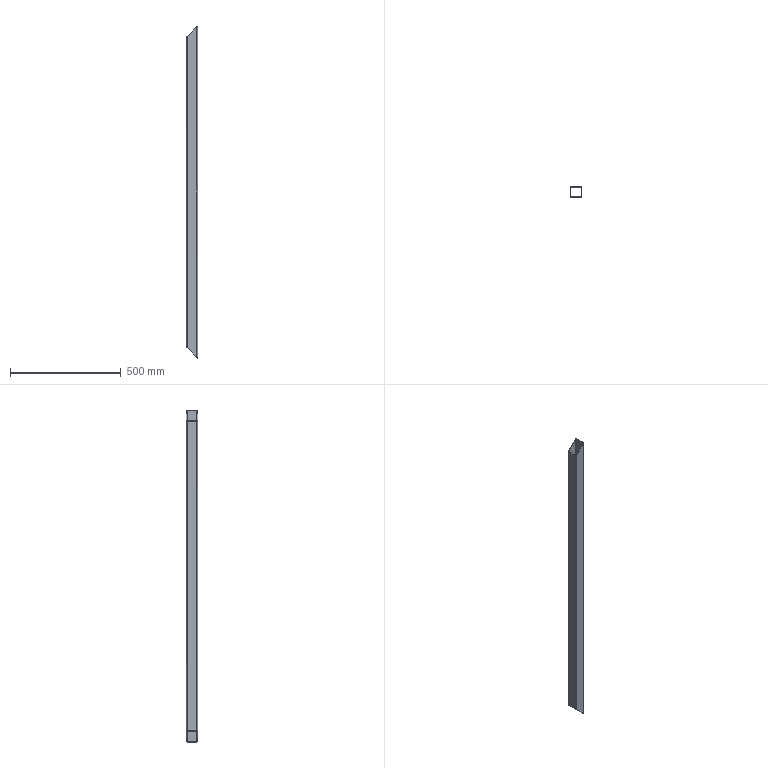Part | SolidWorks | features BaseBody 1 | 1 solid | 18 faces | box 50 x 50 x 1498 mm | volume 541116 mm3 | plane 10 | cylinder 8 | commonest cylinder face diameters 4 x4 8 x4
STEP:
#1=CARTESIAN_POINT('',(-25.,21.,699.));
#2=VERTEX_POINT('',#1);
#3=CARTESIAN_POINT('',(-25.,21.,-699.));
#4=VERTEX_POINT('',#3);
#5=CARTESIAN_POINT('',(-25.,21.,749.));
#6=DIRECTION('',(0.,0.,-1.));
#7=VECTOR('',#6,1000.);
#8=LINE('',#5,#7);
#9=EDGE_CURVE('',#2,#4,#8,.T.);
#10=ORIENTED_EDGE('',*,*,#9,.T.);
#11=CARTESIAN_POINT('',(-25.,-21.,-699.));
#12=VERTEX_POINT('',#11);
#13=CARTESIAN_POINT('',(-25.,-25.,-699.));
#14=DIRECTION('',(0.,1.,0.));
#15=VECTOR('',#14,1000.);
#16=LINE('',#13,#15);
#17=EDGE_CURVE('',#12,#4,#16,.T.);
#18=ORIENTED_EDGE('',*,*,#17,.F.);
#19=CARTESIAN_POINT('',(-25.,-21.,699.));
#20=VERTEX_POINT('',#19);
#21=CARTESIAN_POINT('',(-25.,-21.,749.));
#22=DIRECTION('',(0.,0.,-1.));
#23=VECTOR('',#22,1000.);
#24=LINE('',#21,#23);
#25=EDGE_CURVE('',#20,#12,#24,.T.);
#26=ORIENTED_EDGE('',*,*,#25,.F.);
#27=CARTESIAN_POINT('',(-25.,-25.,699.));
#28=DIRECTION('',(0.,1.,0.));
#29=VECTOR('',#28,1000.);
#30=LINE('',#27,#29);
#31=EDGE_CURVE('',#20,#2,#30,.T.);
#32=ORIENTED_EDGE('',*,*,#31,.T.);
#33=EDGE_LOOP('',(#10,#18,#26,#32));
#34=FACE_OUTER_BOUND('',#33,.T.);
#35=CARTESIAN_POINT('',(-25.,21.,749.));
#36=DIRECTION('',(1.,0.,0.));
#37=DIRECTION('',(0.,1.,0.));
#38=AXIS2_PLACEMENT_3D('',#35,#36,#37);
#39=PLANE('',#38);
#40=ADVANCED_FACE('',(#34),#39,.F.);
#41=CARTESIAN_POINT('',(-21.,25.,703.));
#42=VERTEX_POINT('',#41);
#43=CARTESIAN_POINT('',(-21.,25.,-703.));
#44=VERTEX_POINT('',#43);
#45=CARTESIAN_POINT('',(-21.,25.,749.));
#46=DIRECTION('',(0.,0.,-1.));
#47=VECTOR('',#46,1000.);
#48=LINE('',#45,#47);
#49=EDGE_CURVE('',#42,#44,#48,.T.);
#50=ORIENTED_EDGE('',*,*,#49,.T.);
#51=CARTESIAN_POINT('',(-21.,25.,-703.));
#52=CARTESIAN_POINT('',(-23.343,25.,-700.657));
#53=CARTESIAN_POINT('',(-25.,23.343,-699.));
#54=CARTESIAN_POINT('',(-25.,21.,-699.));
#55=(BOUNDED_CURVE()B_SPLINE_CURVE(3,(#51,#52,#53,#54),.UNSPECIFIED.,.F.,.F.)B_SPLINE_CURVE_WITH_KNOTS((4,4),(1.571,3.142),.UNSPECIFIED.)CURVE()GEOMETRIC_REPRESENTATION_ITEM()RATIONAL_B_SPLINE_CURVE((1.,0.8047,0.8047,1.))REPRESENTATION_ITEM(''));
#56=EDGE_CURVE('',#44,#4,#55,.T.);
#57=ORIENTED_EDGE('',*,*,#56,.T.);
#58=ORIENTED_EDGE('',*,*,#9,.F.);
#59=CARTESIAN_POINT('',(-25.,21.,699.));
#60=CARTESIAN_POINT('',(-25.,23.343,699.));
#61=CARTESIAN_POINT('',(-23.343,25.,700.657));
#62=CARTESIAN_POINT('',(-21.,25.,703.));
#63=(BOUNDED_CURVE()B_SPLINE_CURVE(3,(#59,#60,#61,#62),.UNSPECIFIED.,.F.,.F.)B_SPLINE_CURVE_WITH_KNOTS((4,4),(0.,1.571),.UNSPECIFIED.)CURVE()GEOMETRIC_REPRESENTATION_ITEM()RATIONAL_B_SPLINE_CURVE((1.,0.8047,0.8047,1.))REPRESENTATION_ITEM(''));
#64=EDGE_CURVE('',#2,#42,#63,.T.);
#65=ORIENTED_EDGE('',*,*,#64,.T.);
#66=EDGE_LOOP('',(#50,#57,#58,#65));
#67=FACE_OUTER_BOUND('',#66,.T.);
#68=CARTESIAN_POINT('',(-21.,21.,749.));
#69=DIRECTION('',(0.,0.,-1.));
#70=DIRECTION('',(-1.,0.,0.));
#71=AXIS2_PLACEMENT_3D('',#68,#69,#70);
#72=CYLINDRICAL_SURFACE('',#71,4.);
#73=ADVANCED_FACE('',(#67),#72,.T.);
#74=CARTESIAN_POINT('',(21.,25.,745.));
#75=VERTEX_POINT('',#74);
#76=CARTESIAN_POINT('',(21.,25.,-745.));
#77=VERTEX_POINT('',#76);
#78=CARTESIAN_POINT('',(21.,25.,749.));
#79=DIRECTION('',(0.,0.,-1.));
#80=VECTOR('',#79,1000.);
#81=LINE('',#78,#80);
#82=EDGE_CURVE('',#75,#77,#81,.T.);
#83=ORIENTED_EDGE('',*,*,#82,.T.);
#84=CARTESIAN_POINT('',(25.,25.,-749.));
#85=DIRECTION('',(0.7071,0.,-0.7071));
#86=VECTOR('',#85,1000.);
#87=LINE('',#84,#86);
#88=EDGE_CURVE('',#44,#77,#87,.T.);
#89=ORIENTED_EDGE('',*,*,#88,.F.);
#90=ORIENTED_EDGE('',*,*,#49,.F.);
#91=CARTESIAN_POINT('',(25.,25.,749.));
#92=DIRECTION('',(-0.7071,0.,-0.7071));
#93=VECTOR('',#92,1000.);
#94=LINE('',#91,#93);
#95=EDGE_CURVE('',#75,#42,#94,.T.);
#96=ORIENTED_EDGE('',*,*,#95,.F.);
#97=EDGE_LOOP('',(#83,#89,#90,#96));
#98=FACE_OUTER_BOUND('',#97,.T.);
#99=CARTESIAN_POINT('',(-21.,25.,749.));
#100=DIRECTION('',(0.,-1.,0.));
#101=DIRECTION('',(0.,0.,-1.));
#102=AXIS2_PLACEMENT_3D('',#99,#100,#101);
#103=PLANE('',#102);
#104=ADVANCED_FACE('',(#98),#103,.F.);
#105=CARTESIAN_POINT('',(25.,21.,749.));
#106=VERTEX_POINT('',#105);
#107=CARTESIAN_POINT('',(25.,21.,-749.));
#108=VERTEX_POINT('',#107);
#109=CARTESIAN_POINT('',(25.,21.,749.));
#110=DIRECTION('',(0.,0.,-1.));
#111=VECTOR('',#110,1000.);
#112=LINE('',#109,#111);
#113=EDGE_CURVE('',#106,#108,#112,.T.);
#114=ORIENTED_EDGE('',*,*,#113,.T.);
#115=CARTESIAN_POINT('',(25.,21.,-749.));
#116=CARTESIAN_POINT('',(25.,23.343,-749.));
#117=CARTESIAN_POINT('',(23.343,25.,-747.343));
#118=CARTESIAN_POINT('',(21.,25.,-745.));
#119=(BOUNDED_CURVE()B_SPLINE_CURVE(3,(#115,#116,#117,#118),.UNSPECIFIED.,.F.,.F.)B_SPLINE_CURVE_WITH_KNOTS((4,4),(0.,1.571),.UNSPECIFIED.)CURVE()GEOMETRIC_REPRESENTATION_ITEM()RATIONAL_B_SPLINE_CURVE((1.,0.8047,0.8047,1.))REPRESENTATION_ITEM(''));
#120=EDGE_CURVE('',#108,#77,#119,.T.);
#121=ORIENTED_EDGE('',*,*,#120,.T.);
#122=ORIENTED_EDGE('',*,*,#82,.F.);
#123=CARTESIAN_POINT('',(21.,25.,745.));
#124=CARTESIAN_POINT('',(23.343,25.,747.343));
#125=CARTESIAN_POINT('',(25.,23.343,749.));
#126=CARTESIAN_POINT('',(25.,21.,749.));
#127=(BOUNDED_CURVE()B_SPLINE_CURVE(3,(#123,#124,#125,#126),.UNSPECIFIED.,.F.,.F.)B_SPLINE_CURVE_WITH_KNOTS((4,4),(1.571,3.142),.UNSPECIFIED.)CURVE()GEOMETRIC_REPRESENTATION_ITEM()RATIONAL_B_SPLINE_CURVE((1.,0.8047,0.8047,1.))REPRESENTATION_ITEM(''));
#128=EDGE_CURVE('',#75,#106,#127,.T.);
#129=ORIENTED_EDGE('',*,*,#128,.T.);
#130=EDGE_LOOP('',(#114,#121,#122,#129));
#131=FACE_OUTER_BOUND('',#130,.T.);
#132=CARTESIAN_POINT('',(21.,21.,749.));
#133=DIRECTION('',(0.,0.,-1.));
#134=DIRECTION('',(-1.,0.,0.));
#135=AXIS2_PLACEMENT_3D('',#132,#133,#134);
#136=CYLINDRICAL_SURFACE('',#135,4.);
#137=ADVANCED_FACE('',(#131),#136,.T.);
#138=CARTESIAN_POINT('',(25.,-21.,-749.));
#139=VERTEX_POINT('',#138);
#140=CARTESIAN_POINT('',(25.,21.,-749.));
#141=DIRECTION('',(0.,1.,0.));
#142=VECTOR('',#141,1000.);
#143=LINE('',#140,#142);
#144=EDGE_CURVE('',#139,#108,#143,.T.);
#145=ORIENTED_EDGE('',*,*,#144,.T.);
#146=ORIENTED_EDGE('',*,*,#113,.F.);
#147=CARTESIAN_POINT('',(25.,-21.,749.));
#148=VERTEX_POINT('',#147);
#149=CARTESIAN_POINT('',(25.,21.,749.));
#150=DIRECTION('',(0.,1.,0.));
#151=VECTOR('',#150,1000.);
#152=LINE('',#149,#151);
#153=EDGE_CURVE('',#148,#106,#152,.T.);
#154=ORIENTED_EDGE('',*,*,#153,.F.);
#155=CARTESIAN_POINT('',(25.,-21.,749.));
#156=DIRECTION('',(0.,0.,-1.));
#157=VECTOR('',#156,1000.);
#158=LINE('',#155,#157);
#159=EDGE_CURVE('',#148,#139,#158,.T.);
#160=ORIENTED_EDGE('',*,*,#159,.T.);
#161=EDGE_LOOP('',(#145,#146,#154,#160));
#162=FACE_OUTER_BOUND('',#161,.T.);
#163=CARTESIAN_POINT('',(25.,21.,749.));
#164=DIRECTION('',(-1.,0.,0.));
#165=DIRECTION('',(0.,1.,0.));
#166=AXIS2_PLACEMENT_3D('',#163,#164,#165);
#167=PLANE('',#166);
#168=ADVANCED_FACE('',(#162),#167,.F.);
#169=CARTESIAN_POINT('',(21.,-25.,745.));
#170=VERTEX_POINT('',#169);
#171=CARTESIAN_POINT('',(21.,-25.,-745.));
#172=VERTEX_POINT('',#171);
#173=CARTESIAN_POINT('',(21.,-25.,749.));
#174=DIRECTION('',(0.,0.,-1.));
#175=VECTOR('',#174,1000.);
#176=LINE('',#173,#175);
#177=EDGE_CURVE('',#170,#172,#176,.T.);
#178=ORIENTED_EDGE('',*,*,#177,.T.);
#179=CARTESIAN_POINT('',(21.,-25.,-745.));
#180=CARTESIAN_POINT('',(23.343,-25.,-747.343));
#181=CARTESIAN_POINT('',(25.,-23.343,-749.));
#182=CARTESIAN_POINT('',(25.,-21.,-749.));
#183=(BOUNDED_CURVE()B_SPLINE_CURVE(3,(#179,#180,#181,#182),.UNSPECIFIED.,.F.,.T.)B_SPLINE_CURVE_WITH_KNOTS((4,4),(4.712,6.283),.UNSPECIFIED.)CURVE()GEOMETRIC_REPRESENTATION_ITEM()RATIONAL_B_SPLINE_CURVE((1.,0.8047,0.8047,1.))REPRESENTATION_ITEM(''));
#184=EDGE_CURVE('',#172,#139,#183,.T.);
#185=ORIENTED_EDGE('',*,*,#184,.T.);
#186=ORIENTED_EDGE('',*,*,#159,.F.);
#187=CARTESIAN_POINT('',(25.,-21.,749.));
#188=CARTESIAN_POINT('',(25.,-23.343,749.));
#189=CARTESIAN_POINT('',(23.343,-25.,747.343));
#190=CARTESIAN_POINT('',(21.,-25.,745.));
#191=(BOUNDED_CURVE()B_SPLINE_CURVE(3,(#187,#188,#189,#190),.UNSPECIFIED.,.F.,.T.)B_SPLINE_CURVE_WITH_KNOTS((4,4),(3.142,4.712),.UNSPECIFIED.)CURVE()GEOMETRIC_REPRESENTATION_ITEM()RATIONAL_B_SPLINE_CURVE((1.,0.8047,0.8047,1.))REPRESENTATION_ITEM(''));
#192=EDGE_CURVE('',#148,#170,#191,.T.);
#193=ORIENTED_EDGE('',*,*,#192,.T.);
#194=EDGE_LOOP('',(#178,#185,#186,#193));
#195=FACE_OUTER_BOUND('',#194,.T.);
#196=CARTESIAN_POINT('',(21.,-21.,749.));
#197=DIRECTION('',(0.,0.,-1.));
#198=DIRECTION('',(-1.,0.,0.));
#199=AXIS2_PLACEMENT_3D('',#196,#197,#198);
#200=CYLINDRICAL_SURFACE('',#199,4.);
#201=ADVANCED_FACE('',(#195),#200,.T.);
#202=CARTESIAN_POINT('',(-21.,-25.,703.));
#203=VERTEX_POINT('',#202);
#204=CARTESIAN_POINT('',(-21.,-25.,-703.));
#205=VERTEX_POINT('',#204);
#206=CARTESIAN_POINT('',(-21.,-25.,749.));
#207=DIRECTION('',(0.,0.,-1.));
#208=VECTOR('',#207,1000.);
#209=LINE('',#206,#208);
#210=EDGE_CURVE('',#203,#205,#209,.T.);
#211=ORIENTED_EDGE('',*,*,#210,.T.);
#212=CARTESIAN_POINT('',(25.,-25.,-749.));
#213=DIRECTION('',(0.7071,0.,-0.7071));
#214=VECTOR('',#213,1000.);
#215=LINE('',#212,#214);
#216=EDGE_CURVE('',#205,#172,#215,.T.);
#217=ORIENTED_EDGE('',*,*,#216,.T.);
#218=ORIENTED_EDGE('',*,*,#177,.F.);
#219=CARTESIAN_POINT('',(25.,-25.,749.));
#220=DIRECTION('',(-0.7071,0.,-0.7071));
#221=VECTOR('',#220,1000.);
#222=LINE('',#219,#221);
#223=EDGE_CURVE('',#170,#203,#222,.T.);
#224=ORIENTED_EDGE('',*,*,#223,.T.);
#225=EDGE_LOOP('',(#211,#217,#218,#224));
#226=FACE_OUTER_BOUND('',#225,.T.);
#227=CARTESIAN_POINT('',(-21.,-25.,749.));
#228=DIRECTION('',(0.,1.,0.));
#229=DIRECTION('',(1.,0.,0.));
#230=AXIS2_PLACEMENT_3D('',#227,#228,#229);
#231=PLANE('',#230);
#232=ADVANCED_FACE('',(#226),#231,.F.);
#233=ORIENTED_EDGE('',*,*,#25,.T.);
#234=CARTESIAN_POINT('',(-25.,-21.,-699.));
#235=CARTESIAN_POINT('',(-25.,-23.343,-699.));
#236=CARTESIAN_POINT('',(-23.343,-25.,-700.657));
#237=CARTESIAN_POINT('',(-21.,-25.,-703.));
#238=(BOUNDED_CURVE()B_SPLINE_CURVE(3,(#234,#235,#236,#237),.UNSPECIFIED.,.F.,.F.)B_SPLINE_CURVE_WITH_KNOTS((4,4),(3.142,4.712),.UNSPECIFIED.)CURVE()GEOMETRIC_REPRESENTATION_ITEM()RATIONAL_B_SPLINE_CURVE((1.,0.8047,0.8047,1.))REPRESENTATION_ITEM(''));
#239=EDGE_CURVE('',#12,#205,#238,.T.);
#240=ORIENTED_EDGE('',*,*,#239,.T.);
#241=ORIENTED_EDGE('',*,*,#210,.F.);
#242=CARTESIAN_POINT('',(-21.,-25.,703.));
#243=CARTESIAN_POINT('',(-23.343,-25.,700.657));
#244=CARTESIAN_POINT('',(-25.,-23.343,699.));
#245=CARTESIAN_POINT('',(-25.,-21.,699.));
#246=(BOUNDED_CURVE()B_SPLINE_CURVE(3,(#242,#243,#244,#245),.UNSPECIFIED.,.F.,.T.)B_SPLINE_CURVE_WITH_KNOTS((4,4),(4.712,6.283),.UNSPECIFIED.)CURVE()GEOMETRIC_REPRESENTATION_ITEM()RATIONAL_B_SPLINE_CURVE((1.,0.8047,0.8047,1.))REPRESENTATION_ITEM(''));
#247=EDGE_CURVE('',#203,#20,#246,.T.);
#248=ORIENTED_EDGE('',*,*,#247,.T.);
#249=EDGE_LOOP('',(#233,#240,#241,#248));
#250=FACE_OUTER_BOUND('',#249,.T.);
#251=CARTESIAN_POINT('',(-21.,-21.,749.));
#252=DIRECTION('',(0.,0.,-1.));
#253=DIRECTION('',(-1.,0.,0.));
#254=AXIS2_PLACEMENT_3D('',#251,#252,#253);
#255=CYLINDRICAL_SURFACE('',#254,4.);
#256=ADVANCED_FACE('',(#250),#255,.T.);
#257=CARTESIAN_POINT('',(-23.,-21.,-701.));
#258=VERTEX_POINT('',#257);
#259=CARTESIAN_POINT('',(-21.,-23.,-703.));
#260=VERTEX_POINT('',#259);
#261=CARTESIAN_POINT('',(-23.,-21.,-701.));
#262=CARTESIAN_POINT('',(-23.,-22.172,-701.));
#263=CARTESIAN_POINT('',(-22.172,-23.,-701.828));
#264=CARTESIAN_POINT('',(-21.,-23.,-703.));
#265=(BOUNDED_CURVE()B_SPLINE_CURVE(3,(#261,#262,#263,#264),.UNSPECIFIED.,.F.,.F.)B_SPLINE_CURVE_WITH_KNOTS((4,4),(3.142,4.712),.UNSPECIFIED.)CURVE()GEOMETRIC_REPRESENTATION_ITEM()RATIONAL_B_SPLINE_CURVE((1.,0.8047,0.8047,1.))REPRESENTATION_ITEM(''));
#266=EDGE_CURVE('',#258,#260,#265,.T.);
#267=ORIENTED_EDGE('',*,*,#266,.T.);
#268=CARTESIAN_POINT('',(21.,-23.,-745.));
#269=VERTEX_POINT('',#268);
#270=CARTESIAN_POINT('',(-747.,-23.,23.));
#271=DIRECTION('',(0.7071,0.,-0.7071));
#272=VECTOR('',#271,1000.);
#273=LINE('',#270,#272);
#274=EDGE_CURVE('',#260,#269,#273,.T.);
#275=ORIENTED_EDGE('',*,*,#274,.T.);
#276=CARTESIAN_POINT('',(23.,-21.,-747.));
#277=VERTEX_POINT('',#276);
#278=CARTESIAN_POINT('',(21.,-23.,-745.));
#279=CARTESIAN_POINT('',(22.172,-23.,-746.172));
#280=CARTESIAN_POINT('',(23.,-22.172,-747.));
#281=CARTESIAN_POINT('',(23.,-21.,-747.));
#282=(BOUNDED_CURVE()B_SPLINE_CURVE(3,(#278,#279,#280,#281),.UNSPECIFIED.,.F.,.T.)B_SPLINE_CURVE_WITH_KNOTS((4,4),(4.712,6.283),.UNSPECIFIED.)CURVE()GEOMETRIC_REPRESENTATION_ITEM()RATIONAL_B_SPLINE_CURVE((1.,0.8047,0.8047,1.))REPRESENTATION_ITEM(''));
#283=EDGE_CURVE('',#269,#277,#282,.T.);
#284=ORIENTED_EDGE('',*,*,#283,.T.);
#285=CARTESIAN_POINT('',(23.,21.,-747.));
#286=VERTEX_POINT('',#285);
#287=CARTESIAN_POINT('',(23.,21.,-747.));
#288=DIRECTION('',(0.,1.,0.));
#289=VECTOR('',#288,1000.);
#290=LINE('',#287,#289);
#291=EDGE_CURVE('',#277,#286,#290,.T.);
#292=ORIENTED_EDGE('',*,*,#291,.T.);
#293=CARTESIAN_POINT('',(21.,23.,-745.));
#294=VERTEX_POINT('',#293);
#295=CARTESIAN_POINT('',(23.,21.,-747.));
#296=CARTESIAN_POINT('',(23.,22.172,-747.));
#297=CARTESIAN_POINT('',(22.172,23.,-746.172));
#298=CARTESIAN_POINT('',(21.,23.,-745.));
#299=(BOUNDED_CURVE()B_SPLINE_CURVE(3,(#295,#296,#297,#298),.UNSPECIFIED.,.F.,.F.)B_SPLINE_CURVE_WITH_KNOTS((4,4),(0.,1.571),.UNSPECIFIED.)CURVE()GEOMETRIC_REPRESENTATION_ITEM()RATIONAL_B_SPLINE_CURVE((1.,0.8047,0.8047,1.))REPRESENTATION_ITEM(''));
#300=EDGE_CURVE('',#286,#294,#299,.T.);
#301=ORIENTED_EDGE('',*,*,#300,.T.);
#302=CARTESIAN_POINT('',(-21.,23.,-703.));
#303=VERTEX_POINT('',#302);
#304=CARTESIAN_POINT('',(-747.,23.,23.));
#305=DIRECTION('',(-0.7071,0.,0.7071));
#306=VECTOR('',#305,1000.);
#307=LINE('',#304,#306);
#308=EDGE_CURVE('',#294,#303,#307,.T.);
#309=ORIENTED_EDGE('',*,*,#308,.T.);
#310=CARTESIAN_POINT('',(-23.,21.,-701.));
#311=VERTEX_POINT('',#310);
#312=CARTESIAN_POINT('',(-21.,23.,-703.));
#313=CARTESIAN_POINT('',(-22.172,23.,-701.828));
#314=CARTESIAN_POINT('',(-23.,22.172,-701.));
#315=CARTESIAN_POINT('',(-23.,21.,-701.));
#316=(BOUNDED_CURVE()B_SPLINE_CURVE(3,(#312,#313,#314,#315),.UNSPECIFIED.,.F.,.T.)B_SPLINE_CURVE_WITH_KNOTS((4,4),(1.571,3.142),.UNSPECIFIED.)CURVE()GEOMETRIC_REPRESENTATION_ITEM()RATIONAL_B_SPLINE_CURVE((1.,0.8047,0.8047,1.))REPRESENTATION_ITEM(''));
#317=EDGE_CURVE('',#303,#311,#316,.T.);
#318=ORIENTED_EDGE('',*,*,#317,.T.);
#319=CARTESIAN_POINT('',(-23.,21.,-701.));
#320=DIRECTION('',(0.,-1.,0.));
#321=VECTOR('',#320,1000.);
#322=LINE('',#319,#321);
#323=EDGE_CURVE('',#311,#258,#322,.T.);
#324=ORIENTED_EDGE('',*,*,#323,.T.);
#325=EDGE_LOOP('',(#267,#275,#284,#292,#301,#309,#318,#324));
#326=FACE_BOUND('',#325,.T.);
#327=ORIENTED_EDGE('',*,*,#17,.T.);
#328=ORIENTED_EDGE('',*,*,#56,.F.);
#329=ORIENTED_EDGE('',*,*,#88,.T.);
#330=ORIENTED_EDGE('',*,*,#120,.F.);
#331=ORIENTED_EDGE('',*,*,#144,.F.);
#332=ORIENTED_EDGE('',*,*,#184,.F.);
#333=ORIENTED_EDGE('',*,*,#216,.F.);
#334=ORIENTED_EDGE('',*,*,#239,.F.);
#335=EDGE_LOOP('',(#327,#328,#329,#330,#331,#332,#333,#334));
#336=FACE_OUTER_BOUND('',#335,.T.);
#337=CARTESIAN_POINT('',(25.,-25.,-749.));
#338=DIRECTION('',(0.7071,0.,0.7071));
#339=DIRECTION('',(0.,-1.,0.));
#340=AXIS2_PLACEMENT_3D('',#337,#338,#339);
#341=PLANE('',#340);
#342=ADVANCED_FACE('',(#326,#336),#341,.F.);
#343=CARTESIAN_POINT('',(-21.,-23.,703.));
#344=VERTEX_POINT('',#343);
#345=CARTESIAN_POINT('',(-23.,-21.,701.));
#346=VERTEX_POINT('',#345);
#347=CARTESIAN_POINT('',(-21.,-23.,703.));
#348=CARTESIAN_POINT('',(-22.172,-23.,701.828));
#349=CARTESIAN_POINT('',(-23.,-22.172,701.));
#350=CARTESIAN_POINT('',(-23.,-21.,701.));
#351=(BOUNDED_CURVE()B_SPLINE_CURVE(3,(#347,#348,#349,#350),.UNSPECIFIED.,.F.,.T.)B_SPLINE_CURVE_WITH_KNOTS((4,4),(4.712,6.283),.UNSPECIFIED.)CURVE()GEOMETRIC_REPRESENTATION_ITEM()RATIONAL_B_SPLINE_CURVE((1.,0.8047,0.8047,1.))REPRESENTATION_ITEM(''));
#352=EDGE_CURVE('',#344,#346,#351,.T.);
#353=ORIENTED_EDGE('',*,*,#352,.T.);
#354=CARTESIAN_POINT('',(-23.,21.,701.));
#355=VERTEX_POINT('',#354);
#356=CARTESIAN_POINT('',(-23.,21.,701.));
#357=DIRECTION('',(0.,1.,0.));
#358=VECTOR('',#357,1000.);
#359=LINE('',#356,#358);
#360=EDGE_CURVE('',#346,#355,#359,.T.);
#361=ORIENTED_EDGE('',*,*,#360,.T.);
#362=CARTESIAN_POINT('',(-21.,23.,703.));
#363=VERTEX_POINT('',#362);
#364=CARTESIAN_POINT('',(-23.,21.,701.));
#365=CARTESIAN_POINT('',(-23.,22.172,701.));
#366=CARTESIAN_POINT('',(-22.172,23.,701.828));
#367=CARTESIAN_POINT('',(-21.,23.,703.));
#368=(BOUNDED_CURVE()B_SPLINE_CURVE(3,(#364,#365,#366,#367),.UNSPECIFIED.,.F.,.F.)B_SPLINE_CURVE_WITH_KNOTS((4,4),(0.,1.571),.UNSPECIFIED.)CURVE()GEOMETRIC_REPRESENTATION_ITEM()RATIONAL_B_SPLINE_CURVE((1.,0.8047,0.8047,1.))REPRESENTATION_ITEM(''));
#369=EDGE_CURVE('',#355,#363,#368,.T.);
#370=ORIENTED_EDGE('',*,*,#369,.T.);
#371=CARTESIAN_POINT('',(21.,23.,745.));
#372=VERTEX_POINT('',#371);
#373=CARTESIAN_POINT('',(2.,23.,726.));
#374=DIRECTION('',(0.7071,0.,0.7071));
#375=VECTOR('',#374,1000.);
#376=LINE('',#373,#375);
#377=EDGE_CURVE('',#363,#372,#376,.T.);
#378=ORIENTED_EDGE('',*,*,#377,.T.);
#379=CARTESIAN_POINT('',(23.,21.,747.));
#380=VERTEX_POINT('',#379);
#381=CARTESIAN_POINT('',(21.,23.,745.));
#382=CARTESIAN_POINT('',(22.172,23.,746.172));
#383=CARTESIAN_POINT('',(23.,22.172,747.));
#384=CARTESIAN_POINT('',(23.,21.,747.));
#385=(BOUNDED_CURVE()B_SPLINE_CURVE(3,(#381,#382,#383,#384),.UNSPECIFIED.,.F.,.T.)B_SPLINE_CURVE_WITH_KNOTS((4,4),(1.571,3.142),.UNSPECIFIED.)CURVE()GEOMETRIC_REPRESENTATION_ITEM()RATIONAL_B_SPLINE_CURVE((1.,0.8047,0.8047,1.))REPRESENTATION_ITEM(''));
#386=EDGE_CURVE('',#372,#380,#385,.T.);
#387=ORIENTED_EDGE('',*,*,#386,.T.);
#388=CARTESIAN_POINT('',(23.,-21.,747.));
#389=VERTEX_POINT('',#388);
#390=CARTESIAN_POINT('',(23.,21.,747.));
#391=DIRECTION('',(0.,-1.,0.));
#392=VECTOR('',#391,1000.);
#393=LINE('',#390,#392);
#394=EDGE_CURVE('',#380,#389,#393,.T.);
#395=ORIENTED_EDGE('',*,*,#394,.T.);
#396=CARTESIAN_POINT('',(21.,-23.,745.));
#397=VERTEX_POINT('',#396);
#398=CARTESIAN_POINT('',(23.,-21.,747.));
#399=CARTESIAN_POINT('',(23.,-22.172,747.));
#400=CARTESIAN_POINT('',(22.172,-23.,746.172));
#401=CARTESIAN_POINT('',(21.,-23.,745.));
#402=(BOUNDED_CURVE()B_SPLINE_CURVE(3,(#398,#399,#400,#401),.UNSPECIFIED.,.F.,.F.)B_SPLINE_CURVE_WITH_KNOTS((4,4),(3.142,4.712),.UNSPECIFIED.)CURVE()GEOMETRIC_REPRESENTATION_ITEM()RATIONAL_B_SPLINE_CURVE((1.,0.8047,0.8047,1.))REPRESENTATION_ITEM(''));
#403=EDGE_CURVE('',#389,#397,#402,.T.);
#404=ORIENTED_EDGE('',*,*,#403,.T.);
#405=CARTESIAN_POINT('',(2.,-23.,726.));
#406=DIRECTION('',(-0.7071,0.,-0.7071));
#407=VECTOR('',#406,1000.);
#408=LINE('',#405,#407);
#409=EDGE_CURVE('',#397,#344,#408,.T.);
#410=ORIENTED_EDGE('',*,*,#409,.T.);
#411=EDGE_LOOP('',(#353,#361,#370,#378,#387,#395,#404,#410));
#412=FACE_BOUND('',#411,.T.);
#413=ORIENTED_EDGE('',*,*,#223,.F.);
#414=ORIENTED_EDGE('',*,*,#192,.F.);
#415=ORIENTED_EDGE('',*,*,#153,.T.);
#416=ORIENTED_EDGE('',*,*,#128,.F.);
#417=ORIENTED_EDGE('',*,*,#95,.T.);
#418=ORIENTED_EDGE('',*,*,#64,.F.);
#419=ORIENTED_EDGE('',*,*,#31,.F.);
#420=ORIENTED_EDGE('',*,*,#247,.F.);
#421=EDGE_LOOP('',(#413,#414,#415,#416,#417,#418,#419,#420));
#422=FACE_OUTER_BOUND('',#421,.T.);
#423=CARTESIAN_POINT('',(25.,-25.,749.));
#424=DIRECTION('',(0.7071,0.,-0.7071));
#425=DIRECTION('',(0.,-1.,0.));
#426=AXIS2_PLACEMENT_3D('',#423,#424,#425);
#427=PLANE('',#426);
#428=ADVANCED_FACE('',(#412,#422),#427,.F.);
#429=ORIENTED_EDGE('',*,*,#266,.F.);
#430=CARTESIAN_POINT('',(-23.,-21.,749.));
#431=DIRECTION('',(0.,0.,-1.));
#432=VECTOR('',#431,1000.);
#433=LINE('',#430,#432);
#434=EDGE_CURVE('',#346,#258,#433,.T.);
#435=ORIENTED_EDGE('',*,*,#434,.F.);
#436=ORIENTED_EDGE('',*,*,#352,.F.);
#437=CARTESIAN_POINT('',(-21.,-23.,749.));
#438=DIRECTION('',(0.,0.,-1.));
#439=VECTOR('',#438,1000.);
#440=LINE('',#437,#439);
#441=EDGE_CURVE('',#344,#260,#440,.T.);
#442=ORIENTED_EDGE('',*,*,#441,.T.);
#443=EDGE_LOOP('',(#429,#435,#436,#442));
#444=FACE_OUTER_BOUND('',#443,.T.);
#445=CARTESIAN_POINT('',(-21.,-21.,749.));
#446=DIRECTION('',(0.,0.,-1.));
#447=DIRECTION('',(-1.,0.,0.));
#448=AXIS2_PLACEMENT_3D('',#445,#446,#447);
#449=CYLINDRICAL_SURFACE('',#448,2.);
#450=ADVANCED_FACE('',(#444),#449,.F.);
#451=ORIENTED_EDGE('',*,*,#274,.F.);
#452=ORIENTED_EDGE('',*,*,#441,.F.);
#453=ORIENTED_EDGE('',*,*,#409,.F.);
#454=CARTESIAN_POINT('',(21.,-23.,749.));
#455=DIRECTION('',(0.,0.,-1.));
#456=VECTOR('',#455,1000.);
#457=LINE('',#454,#456);
#458=EDGE_CURVE('',#397,#269,#457,.T.);
#459=ORIENTED_EDGE('',*,*,#458,.T.);
#460=EDGE_LOOP('',(#451,#452,#453,#459));
#461=FACE_OUTER_BOUND('',#460,.T.);
#462=CARTESIAN_POINT('',(-21.,-23.,749.));
#463=DIRECTION('',(0.,1.,0.));
#464=DIRECTION('',(1.,0.,0.));
#465=AXIS2_PLACEMENT_3D('',#462,#463,#464);
#466=PLANE('',#465);
#467=ADVANCED_FACE('',(#461),#466,.T.);
#468=ORIENTED_EDGE('',*,*,#283,.F.);
#469=ORIENTED_EDGE('',*,*,#458,.F.);
#470=ORIENTED_EDGE('',*,*,#403,.F.);
#471=CARTESIAN_POINT('',(23.,-21.,749.));
#472=DIRECTION('',(0.,0.,-1.));
#473=VECTOR('',#472,1000.);
#474=LINE('',#471,#473);
#475=EDGE_CURVE('',#389,#277,#474,.T.);
#476=ORIENTED_EDGE('',*,*,#475,.T.);
#477=EDGE_LOOP('',(#468,#469,#470,#476));
#478=FACE_OUTER_BOUND('',#477,.T.);
#479=CARTESIAN_POINT('',(21.,-21.,749.));
#480=DIRECTION('',(0.,0.,-1.));
#481=DIRECTION('',(-1.,0.,0.));
#482=AXIS2_PLACEMENT_3D('',#479,#480,#481);
#483=CYLINDRICAL_SURFACE('',#482,2.);
#484=ADVANCED_FACE('',(#478),#483,.F.);
#485=ORIENTED_EDGE('',*,*,#291,.F.);
#486=ORIENTED_EDGE('',*,*,#475,.F.);
#487=ORIENTED_EDGE('',*,*,#394,.F.);
#488=CARTESIAN_POINT('',(23.,21.,749.));
#489=DIRECTION('',(0.,0.,-1.));
#490=VECTOR('',#489,1000.);
#491=LINE('',#488,#490);
#492=EDGE_CURVE('',#380,#286,#491,.T.);
#493=ORIENTED_EDGE('',*,*,#492,.T.);
#494=EDGE_LOOP('',(#485,#486,#487,#493));
#495=FACE_OUTER_BOUND('',#494,.T.);
#496=CARTESIAN_POINT('',(23.,21.,749.));
#497=DIRECTION('',(-1.,0.,0.));
#498=DIRECTION('',(0.,1.,0.));
#499=AXIS2_PLACEMENT_3D('',#496,#497,#498);
#500=PLANE('',#499);
#501=ADVANCED_FACE('',(#495),#500,.T.);
#502=ORIENTED_EDGE('',*,*,#300,.F.);
#503=ORIENTED_EDGE('',*,*,#492,.F.);
#504=ORIENTED_EDGE('',*,*,#386,.F.);
#505=CARTESIAN_POINT('',(21.,23.,749.));
#506=DIRECTION('',(0.,0.,-1.));
#507=VECTOR('',#506,1000.);
#508=LINE('',#505,#507);
#509=EDGE_CURVE('',#372,#294,#508,.T.);
#510=ORIENTED_EDGE('',*,*,#509,.T.);
#511=EDGE_LOOP('',(#502,#503,#504,#510));
#512=FACE_OUTER_BOUND('',#511,.T.);
#513=CARTESIAN_POINT('',(21.,21.,749.));
#514=DIRECTION('',(0.,0.,-1.));
#515=DIRECTION('',(-1.,0.,0.));
#516=AXIS2_PLACEMENT_3D('',#513,#514,#515);
#517=CYLINDRICAL_SURFACE('',#516,2.);
#518=ADVANCED_FACE('',(#512),#517,.F.);
#519=ORIENTED_EDGE('',*,*,#308,.F.);
#520=ORIENTED_EDGE('',*,*,#509,.F.);
#521=ORIENTED_EDGE('',*,*,#377,.F.);
#522=CARTESIAN_POINT('',(-21.,23.,749.));
#523=DIRECTION('',(0.,0.,-1.));
#524=VECTOR('',#523,1000.);
#525=LINE('',#522,#524);
#526=EDGE_CURVE('',#363,#303,#525,.T.);
#527=ORIENTED_EDGE('',*,*,#526,.T.);
#528=EDGE_LOOP('',(#519,#520,#521,#527));
#529=FACE_OUTER_BOUND('',#528,.T.);
#530=CARTESIAN_POINT('',(-21.,23.,749.));
#531=DIRECTION('',(0.,-1.,0.));
#532=DIRECTION('',(0.,0.,-1.));
#533=AXIS2_PLACEMENT_3D('',#530,#531,#532);
#534=PLANE('',#533);
#535=ADVANCED_FACE('',(#529),#534,.T.);
#536=ORIENTED_EDGE('',*,*,#317,.F.);
#537=ORIENTED_EDGE('',*,*,#526,.F.);
#538=ORIENTED_EDGE('',*,*,#369,.F.);
#539=CARTESIAN_POINT('',(-23.,21.,749.));
#540=DIRECTION('',(0.,0.,-1.));
#541=VECTOR('',#540,1000.);
#542=LINE('',#539,#541);
#543=EDGE_CURVE('',#355,#311,#542,.T.);
#544=ORIENTED_EDGE('',*,*,#543,.T.);
#545=EDGE_LOOP('',(#536,#537,#538,#544));
#546=FACE_OUTER_BOUND('',#545,.T.);
#547=CARTESIAN_POINT('',(-21.,21.,749.));
#548=DIRECTION('',(0.,0.,-1.));
#549=DIRECTION('',(-1.,0.,0.));
#550=AXIS2_PLACEMENT_3D('',#547,#548,#549);
#551=CYLINDRICAL_SURFACE('',#550,2.);
#552=ADVANCED_FACE('',(#546),#551,.F.);
#553=ORIENTED_EDGE('',*,*,#323,.F.);
#554=ORIENTED_EDGE('',*,*,#543,.F.);
#555=ORIENTED_EDGE('',*,*,#360,.F.);
#556=ORIENTED_EDGE('',*,*,#434,.T.);
#557=EDGE_LOOP('',(#553,#554,#555,#556));
#558=FACE_OUTER_BOUND('',#557,.T.);
#559=CARTESIAN_POINT('',(-23.,21.,749.));
#560=DIRECTION('',(1.,0.,0.));
#561=DIRECTION('',(0.,1.,0.));
#562=AXIS2_PLACEMENT_3D('',#559,#560,#561);
#563=PLANE('',#562);
#564=ADVANCED_FACE('',(#558),#563,.T.);
#565=CLOSED_SHELL('',(#40,#73,#104,#137,#168,#201,#232,#256,#342,#428,#450,#467,#484,#501,#518,#535,#552,#564));
#566=MANIFOLD_SOLID_BREP('',#565);
#567=CARTESIAN_POINT('',(0.,0.,0.));
#568=DIRECTION('',(0.,0.,1.));
#569=DIRECTION('',(1.,0.,0.));
#570=AXIS2_PLACEMENT_3D('',#567,#568,#569);
#571=(LENGTH_UNIT()NAMED_UNIT(*)SI_UNIT(.MILLI.,.METRE.));
#572=UNCERTAINTY_MEASURE_WITH_UNIT(LENGTH_MEASURE(0.00001),#571,'','');
#573=(NAMED_UNIT(*)PLANE_ANGLE_UNIT()SI_UNIT($,.RADIAN.));
#574=(NAMED_UNIT(*)SI_UNIT($,.STERADIAN.)SOLID_ANGLE_UNIT());
#575=(GEOMETRIC_REPRESENTATION_CONTEXT(3)GLOBAL_UNCERTAINTY_ASSIGNED_CONTEXT((#572))GLOBAL_UNIT_ASSIGNED_CONTEXT((#571,#573,#574))REPRESENTATION_CONTEXT('',''));
#576=ADVANCED_BREP_SHAPE_REPRESENTATION('',(#566,#570),#575);